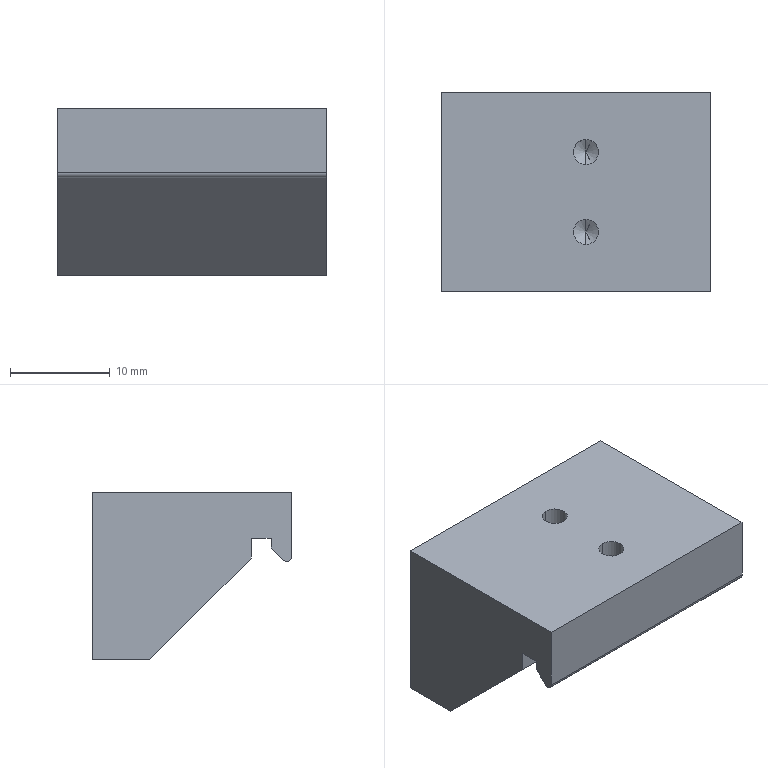Part | NX | 1 solid | 20 faces | box 27 x 20 x 16.8 mm | volume 6363 mm3 | plane 11 | cylinder 5 | cone 4 | commonest cylinder face diameters 2.5 x4 1 x1
STEP:
#1=CARTESIAN_POINT('',(1.,-5.25,-6.749));
#2=VERTEX_POINT('',#1);
#3=CARTESIAN_POINT('',(1.,-2.75,-6.749));
#4=VERTEX_POINT('',#3);
#5=CARTESIAN_POINT('',(1.,-4.,-6.749));
#6=DIRECTION('',(0.,0.,1.));
#7=DIRECTION('',(0.,1.,0.));
#8=AXIS2_PLACEMENT_3D('',#5,#6,#7);
#9=CIRCLE('',#8,1.25);
#10=EDGE_CURVE('',#2,#4,#9,.T.);
#11=ORIENTED_EDGE('',*,*,#10,.F.);
#12=CARTESIAN_POINT('',(1.,-5.25,0.));
#13=VERTEX_POINT('',#12);
#14=CARTESIAN_POINT('',(1.,-5.25,0.));
#15=DIRECTION('',(0.,0.,1.));
#16=VECTOR('',#15,1000.);
#17=LINE('',#14,#16);
#18=EDGE_CURVE('',#13,#2,#17,.F.);
#19=ORIENTED_EDGE('',*,*,#18,.F.);
#20=CARTESIAN_POINT('',(1.,-2.75,0.));
#21=VERTEX_POINT('',#20);
#22=CARTESIAN_POINT('',(1.,-4.,0.));
#23=DIRECTION('',(0.,0.,1.));
#24=DIRECTION('',(0.,1.,0.));
#25=AXIS2_PLACEMENT_3D('',#22,#23,#24);
#26=CIRCLE('',#25,1.25);
#27=EDGE_CURVE('',#13,#21,#26,.T.);
#28=ORIENTED_EDGE('',*,*,#27,.T.);
#29=CARTESIAN_POINT('',(1.,-2.75,0.));
#30=DIRECTION('',(0.,0.,1.));
#31=VECTOR('',#30,1000.);
#32=LINE('',#29,#31);
#33=EDGE_CURVE('',#21,#4,#32,.F.);
#34=ORIENTED_EDGE('',*,*,#33,.T.);
#35=EDGE_LOOP('',(#11,#19,#28,#34));
#36=FACE_BOUND('',#35,.T.);
#37=CARTESIAN_POINT('',(1.,-4.,0.));
#38=DIRECTION('',(0.,0.,1.));
#39=DIRECTION('',(0.,-1.,0.));
#40=AXIS2_PLACEMENT_3D('',#37,#38,#39);
#41=CYLINDRICAL_SURFACE('',#40,1.25);
#42=ADVANCED_FACE('',(#36),#41,.F.);
#43=CARTESIAN_POINT('',(1.,-4.,-7.5));
#44=VERTEX_POINT('',#43);
#45=CARTESIAN_POINT('',(1.,-2.75,-6.749));
#46=DIRECTION('',(0.,0.8572,0.515));
#47=VECTOR('',#46,1000.);
#48=LINE('',#45,#47);
#49=EDGE_CURVE('',#4,#44,#48,.F.);
#50=ORIENTED_EDGE('',*,*,#49,.T.);
#51=CARTESIAN_POINT('',(1.,-5.25,-6.749));
#52=DIRECTION('',(0.,-0.8572,0.515));
#53=VECTOR('',#52,1000.);
#54=LINE('',#51,#53);
#55=EDGE_CURVE('',#2,#44,#54,.F.);
#56=ORIENTED_EDGE('',*,*,#55,.F.);
#57=ORIENTED_EDGE('',*,*,#10,.T.);
#58=EDGE_LOOP('',(#50,#56,#57));
#59=FACE_BOUND('',#58,.T.);
#60=CARTESIAN_POINT('',(1.,-4.,-6.749));
#61=DIRECTION('',(0.,0.,1.));
#62=DIRECTION('',(0.,-1.,0.));
#63=AXIS2_PLACEMENT_3D('',#60,#61,#62);
#64=CONICAL_SURFACE('',#63,1.25,1.03);
#65=ADVANCED_FACE('',(#59),#64,.F.);
#66=CARTESIAN_POINT('',(1.,2.75,-6.749));
#67=VERTEX_POINT('',#66);
#68=CARTESIAN_POINT('',(1.,5.25,-6.749));
#69=VERTEX_POINT('',#68);
#70=CARTESIAN_POINT('',(1.,4.,-6.749));
#71=DIRECTION('',(0.,0.,1.));
#72=DIRECTION('',(0.,1.,0.));
#73=AXIS2_PLACEMENT_3D('',#70,#71,#72);
#74=CIRCLE('',#73,1.25);
#75=EDGE_CURVE('',#67,#69,#74,.T.);
#76=ORIENTED_EDGE('',*,*,#75,.F.);
#77=CARTESIAN_POINT('',(1.,2.75,0.));
#78=VERTEX_POINT('',#77);
#79=CARTESIAN_POINT('',(1.,2.75,0.));
#80=DIRECTION('',(0.,0.,1.));
#81=VECTOR('',#80,1000.);
#82=LINE('',#79,#81);
#83=EDGE_CURVE('',#78,#67,#82,.F.);
#84=ORIENTED_EDGE('',*,*,#83,.F.);
#85=CARTESIAN_POINT('',(1.,5.25,0.));
#86=VERTEX_POINT('',#85);
#87=CARTESIAN_POINT('',(1.,4.,0.));
#88=DIRECTION('',(0.,0.,1.));
#89=DIRECTION('',(0.,1.,0.));
#90=AXIS2_PLACEMENT_3D('',#87,#88,#89);
#91=CIRCLE('',#90,1.25);
#92=EDGE_CURVE('',#78,#86,#91,.T.);
#93=ORIENTED_EDGE('',*,*,#92,.T.);
#94=CARTESIAN_POINT('',(1.,5.25,0.));
#95=DIRECTION('',(0.,0.,1.));
#96=VECTOR('',#95,1000.);
#97=LINE('',#94,#96);
#98=EDGE_CURVE('',#86,#69,#97,.F.);
#99=ORIENTED_EDGE('',*,*,#98,.T.);
#100=EDGE_LOOP('',(#76,#84,#93,#99));
#101=FACE_BOUND('',#100,.T.);
#102=CARTESIAN_POINT('',(1.,4.,0.));
#103=DIRECTION('',(0.,0.,1.));
#104=DIRECTION('',(0.,-1.,0.));
#105=AXIS2_PLACEMENT_3D('',#102,#103,#104);
#106=CYLINDRICAL_SURFACE('',#105,1.25);
#107=ADVANCED_FACE('',(#101),#106,.F.);
#108=CARTESIAN_POINT('',(1.,4.,-7.5));
#109=VERTEX_POINT('',#108);
#110=CARTESIAN_POINT('',(1.,5.25,-6.749));
#111=DIRECTION('',(0.,0.8572,0.515));
#112=VECTOR('',#111,1000.);
#113=LINE('',#110,#112);
#114=EDGE_CURVE('',#69,#109,#113,.F.);
#115=ORIENTED_EDGE('',*,*,#114,.T.);
#116=CARTESIAN_POINT('',(1.,2.75,-6.749));
#117=DIRECTION('',(0.,-0.8572,0.515));
#118=VECTOR('',#117,1000.);
#119=LINE('',#116,#118);
#120=EDGE_CURVE('',#67,#109,#119,.F.);
#121=ORIENTED_EDGE('',*,*,#120,.F.);
#122=ORIENTED_EDGE('',*,*,#75,.T.);
#123=EDGE_LOOP('',(#115,#121,#122));
#124=FACE_BOUND('',#123,.T.);
#125=CARTESIAN_POINT('',(1.,4.,-6.749));
#126=DIRECTION('',(0.,0.,1.));
#127=DIRECTION('',(0.,-1.,0.));
#128=AXIS2_PLACEMENT_3D('',#125,#126,#127);
#129=CONICAL_SURFACE('',#128,1.25,1.03);
#130=ADVANCED_FACE('',(#124),#129,.F.);
#131=CARTESIAN_POINT('',(-13.5,-9.146,-6.816));
#132=VERTEX_POINT('',#131);
#133=CARTESIAN_POINT('',(-13.5,-7.93,-5.6));
#134=VERTEX_POINT('',#133);
#135=CARTESIAN_POINT('',(-13.5,-7.43,-5.1));
#136=DIRECTION('',(0.,0.7071,0.7071));
#137=VECTOR('',#136,1000.);
#138=LINE('',#135,#137);
#139=EDGE_CURVE('',#132,#134,#138,.T.);
#140=ORIENTED_EDGE('',*,*,#139,.F.);
#141=CARTESIAN_POINT('',(-13.5,-10.,-6.463));
#142=VERTEX_POINT('',#141);
#143=CARTESIAN_POINT('',(-13.5,-9.5,-6.463));
#144=DIRECTION('',(-1.,0.,0.));
#145=DIRECTION('',(0.,-1.,0.));
#146=AXIS2_PLACEMENT_3D('',#143,#144,#145);
#147=CIRCLE('',#146,0.5);
#148=EDGE_CURVE('',#132,#142,#147,.T.);
#149=ORIENTED_EDGE('',*,*,#148,.T.);
#150=CARTESIAN_POINT('',(-13.5,-10.,0.));
#151=VERTEX_POINT('',#150);
#152=CARTESIAN_POINT('',(-13.5,-10.,-16.8));
#153=DIRECTION('',(0.,0.,1.));
#154=VECTOR('',#153,1000.);
#155=LINE('',#152,#154);
#156=EDGE_CURVE('',#142,#151,#155,.T.);
#157=ORIENTED_EDGE('',*,*,#156,.T.);
#158=CARTESIAN_POINT('',(-13.5,10.,0.));
#159=VERTEX_POINT('',#158);
#160=CARTESIAN_POINT('',(-13.5,10.,0.));
#161=DIRECTION('',(0.,1.,0.));
#162=VECTOR('',#161,1000.);
#163=LINE('',#160,#162);
#164=EDGE_CURVE('',#151,#159,#163,.T.);
#165=ORIENTED_EDGE('',*,*,#164,.T.);
#166=CARTESIAN_POINT('',(-13.5,10.,-16.8));
#167=VERTEX_POINT('',#166);
#168=CARTESIAN_POINT('',(-13.5,10.,-16.8));
#169=DIRECTION('',(0.,0.,1.));
#170=VECTOR('',#169,1000.);
#171=LINE('',#168,#170);
#172=EDGE_CURVE('',#167,#159,#171,.T.);
#173=ORIENTED_EDGE('',*,*,#172,.F.);
#174=CARTESIAN_POINT('',(-13.5,4.27,-16.8));
#175=VERTEX_POINT('',#174);
#176=CARTESIAN_POINT('',(-13.5,10.,-16.8));
#177=DIRECTION('',(0.,1.,0.));
#178=VECTOR('',#177,1000.);
#179=LINE('',#176,#178);
#180=EDGE_CURVE('',#175,#167,#179,.T.);
#181=ORIENTED_EDGE('',*,*,#180,.F.);
#182=CARTESIAN_POINT('',(-13.5,-5.93,-6.6));
#183=VERTEX_POINT('',#182);
#184=CARTESIAN_POINT('',(-13.5,-7.43,-5.1));
#185=DIRECTION('',(0.,0.7071,-0.7071));
#186=VECTOR('',#185,1000.);
#187=LINE('',#184,#186);
#188=EDGE_CURVE('',#183,#175,#187,.T.);
#189=ORIENTED_EDGE('',*,*,#188,.F.);
#190=CARTESIAN_POINT('',(-13.5,-5.93,-4.6));
#191=VERTEX_POINT('',#190);
#192=CARTESIAN_POINT('',(-13.5,-5.93,-4.6));
#193=DIRECTION('',(0.,0.,-1.));
#194=VECTOR('',#193,1000.);
#195=LINE('',#192,#194);
#196=EDGE_CURVE('',#191,#183,#195,.T.);
#197=ORIENTED_EDGE('',*,*,#196,.F.);
#198=CARTESIAN_POINT('',(-13.5,-7.93,-4.6));
#199=VERTEX_POINT('',#198);
#200=CARTESIAN_POINT('',(-13.5,-7.93,-4.6));
#201=DIRECTION('',(0.,1.,0.));
#202=VECTOR('',#201,1000.);
#203=LINE('',#200,#202);
#204=EDGE_CURVE('',#199,#191,#203,.T.);
#205=ORIENTED_EDGE('',*,*,#204,.F.);
#206=CARTESIAN_POINT('',(-13.5,-7.93,-5.6));
#207=DIRECTION('',(0.,0.,1.));
#208=VECTOR('',#207,1000.);
#209=LINE('',#206,#208);
#210=EDGE_CURVE('',#134,#199,#209,.T.);
#211=ORIENTED_EDGE('',*,*,#210,.F.);
#212=EDGE_LOOP('',(#140,#149,#157,#165,#173,#181,#189,#197,#205,#211));
#213=FACE_BOUND('',#212,.T.);
#214=CARTESIAN_POINT('',(-13.5,10.,-16.8));
#215=DIRECTION('',(1.,0.,0.));
#216=DIRECTION('',(0.,1.,0.));
#217=AXIS2_PLACEMENT_3D('',#214,#215,#216);
#218=PLANE('',#217);
#219=ADVANCED_FACE('',(#213),#218,.F.);
#220=CARTESIAN_POINT('',(13.5,10.,0.));
#221=VERTEX_POINT('',#220);
#222=CARTESIAN_POINT('',(13.5,10.,0.));
#223=DIRECTION('',(1.,0.,0.));
#224=VECTOR('',#223,1000.);
#225=LINE('',#222,#224);
#226=EDGE_CURVE('',#159,#221,#225,.T.);
#227=ORIENTED_EDGE('',*,*,#226,.T.);
#228=CARTESIAN_POINT('',(13.5,10.,-16.8));
#229=VERTEX_POINT('',#228);
#230=CARTESIAN_POINT('',(13.5,10.,-16.8));
#231=DIRECTION('',(0.,0.,1.));
#232=VECTOR('',#231,1000.);
#233=LINE('',#230,#232);
#234=EDGE_CURVE('',#229,#221,#233,.T.);
#235=ORIENTED_EDGE('',*,*,#234,.F.);
#236=CARTESIAN_POINT('',(13.5,10.,-16.8));
#237=DIRECTION('',(1.,0.,0.));
#238=VECTOR('',#237,1000.);
#239=LINE('',#236,#238);
#240=EDGE_CURVE('',#167,#229,#239,.T.);
#241=ORIENTED_EDGE('',*,*,#240,.F.);
#242=ORIENTED_EDGE('',*,*,#172,.T.);
#243=EDGE_LOOP('',(#227,#235,#241,#242));
#244=FACE_BOUND('',#243,.T.);
#245=CARTESIAN_POINT('',(13.5,10.,-16.8));
#246=DIRECTION('',(0.,-1.,0.));
#247=DIRECTION('',(1.,0.,0.));
#248=AXIS2_PLACEMENT_3D('',#245,#246,#247);
#249=PLANE('',#248);
#250=ADVANCED_FACE('',(#244),#249,.F.);
#251=CARTESIAN_POINT('',(13.5,-10.,-6.463));
#252=VERTEX_POINT('',#251);
#253=CARTESIAN_POINT('',(13.5,-10.,0.));
#254=VERTEX_POINT('',#253);
#255=CARTESIAN_POINT('',(13.5,-10.,-16.8));
#256=DIRECTION('',(0.,0.,1.));
#257=VECTOR('',#256,1000.);
#258=LINE('',#255,#257);
#259=EDGE_CURVE('',#252,#254,#258,.T.);
#260=ORIENTED_EDGE('',*,*,#259,.F.);
#261=CARTESIAN_POINT('',(13.5,-9.146,-6.816));
#262=VERTEX_POINT('',#261);
#263=CARTESIAN_POINT('',(13.5,-9.5,-6.463));
#264=DIRECTION('',(1.,0.,0.));
#265=DIRECTION('',(0.,1.,0.));
#266=AXIS2_PLACEMENT_3D('',#263,#264,#265);
#267=CIRCLE('',#266,0.5);
#268=EDGE_CURVE('',#252,#262,#267,.T.);
#269=ORIENTED_EDGE('',*,*,#268,.T.);
#270=CARTESIAN_POINT('',(13.5,-7.93,-5.6));
#271=VERTEX_POINT('',#270);
#272=CARTESIAN_POINT('',(13.5,-7.43,-5.1));
#273=DIRECTION('',(0.,0.7071,0.7071));
#274=VECTOR('',#273,1000.);
#275=LINE('',#272,#274);
#276=EDGE_CURVE('',#262,#271,#275,.T.);
#277=ORIENTED_EDGE('',*,*,#276,.T.);
#278=CARTESIAN_POINT('',(13.5,-7.93,-4.6));
#279=VERTEX_POINT('',#278);
#280=CARTESIAN_POINT('',(13.5,-7.93,-5.6));
#281=DIRECTION('',(0.,0.,1.));
#282=VECTOR('',#281,1000.);
#283=LINE('',#280,#282);
#284=EDGE_CURVE('',#271,#279,#283,.T.);
#285=ORIENTED_EDGE('',*,*,#284,.T.);
#286=CARTESIAN_POINT('',(13.5,-5.93,-4.6));
#287=VERTEX_POINT('',#286);
#288=CARTESIAN_POINT('',(13.5,-7.93,-4.6));
#289=DIRECTION('',(0.,1.,0.));
#290=VECTOR('',#289,1000.);
#291=LINE('',#288,#290);
#292=EDGE_CURVE('',#279,#287,#291,.T.);
#293=ORIENTED_EDGE('',*,*,#292,.T.);
#294=CARTESIAN_POINT('',(13.5,-5.93,-6.6));
#295=VERTEX_POINT('',#294);
#296=CARTESIAN_POINT('',(13.5,-5.93,-16.8));
#297=DIRECTION('',(0.,0.,-1.));
#298=VECTOR('',#297,1000.);
#299=LINE('',#296,#298);
#300=EDGE_CURVE('',#287,#295,#299,.T.);
#301=ORIENTED_EDGE('',*,*,#300,.T.);
#302=CARTESIAN_POINT('',(13.5,4.27,-16.8));
#303=VERTEX_POINT('',#302);
#304=CARTESIAN_POINT('',(13.5,-7.43,-5.1));
#305=DIRECTION('',(0.,0.7071,-0.7071));
#306=VECTOR('',#305,1000.);
#307=LINE('',#304,#306);
#308=EDGE_CURVE('',#295,#303,#307,.T.);
#309=ORIENTED_EDGE('',*,*,#308,.T.);
#310=CARTESIAN_POINT('',(13.5,10.,-16.8));
#311=DIRECTION('',(0.,-1.,0.));
#312=VECTOR('',#311,1000.);
#313=LINE('',#310,#312);
#314=EDGE_CURVE('',#229,#303,#313,.T.);
#315=ORIENTED_EDGE('',*,*,#314,.F.);
#316=ORIENTED_EDGE('',*,*,#234,.T.);
#317=CARTESIAN_POINT('',(13.5,10.,0.));
#318=DIRECTION('',(0.,-1.,0.));
#319=VECTOR('',#318,1000.);
#320=LINE('',#317,#319);
#321=EDGE_CURVE('',#221,#254,#320,.T.);
#322=ORIENTED_EDGE('',*,*,#321,.T.);
#323=EDGE_LOOP('',(#260,#269,#277,#285,#293,#301,#309,#315,#316,#322));
#324=FACE_BOUND('',#323,.T.);
#325=CARTESIAN_POINT('',(13.5,10.,-16.8));
#326=DIRECTION('',(-1.,0.,0.));
#327=DIRECTION('',(0.,-1.,0.));
#328=AXIS2_PLACEMENT_3D('',#325,#326,#327);
#329=PLANE('',#328);
#330=ADVANCED_FACE('',(#324),#329,.F.);
#331=ORIENTED_EDGE('',*,*,#156,.F.);
#332=CARTESIAN_POINT('',(13.5,-10.,-6.463));
#333=DIRECTION('',(1.,0.,0.));
#334=VECTOR('',#333,1000.);
#335=LINE('',#332,#334);
#336=EDGE_CURVE('',#142,#252,#335,.T.);
#337=ORIENTED_EDGE('',*,*,#336,.T.);
#338=ORIENTED_EDGE('',*,*,#259,.T.);
#339=CARTESIAN_POINT('',(13.5,-10.,0.));
#340=DIRECTION('',(-1.,0.,0.));
#341=VECTOR('',#340,1000.);
#342=LINE('',#339,#341);
#343=EDGE_CURVE('',#254,#151,#342,.T.);
#344=ORIENTED_EDGE('',*,*,#343,.T.);
#345=EDGE_LOOP('',(#331,#337,#338,#344));
#346=FACE_BOUND('',#345,.T.);
#347=CARTESIAN_POINT('',(13.5,-10.,-16.8));
#348=DIRECTION('',(0.,1.,0.));
#349=DIRECTION('',(-1.,0.,0.));
#350=AXIS2_PLACEMENT_3D('',#347,#348,#349);
#351=PLANE('',#350);
#352=ADVANCED_FACE('',(#346),#351,.F.);
#353=CARTESIAN_POINT('',(13.5,4.27,-16.8));
#354=DIRECTION('',(-1.,0.,0.));
#355=VECTOR('',#354,1000.);
#356=LINE('',#353,#355);
#357=EDGE_CURVE('',#303,#175,#356,.T.);
#358=ORIENTED_EDGE('',*,*,#357,.T.);
#359=ORIENTED_EDGE('',*,*,#180,.T.);
#360=ORIENTED_EDGE('',*,*,#240,.T.);
#361=ORIENTED_EDGE('',*,*,#314,.T.);
#362=EDGE_LOOP('',(#358,#359,#360,#361));
#363=FACE_BOUND('',#362,.T.);
#364=CARTESIAN_POINT('',(0.,0.,-16.8));
#365=DIRECTION('',(0.,0.,-1.));
#366=DIRECTION('',(0.,1.,0.));
#367=AXIS2_PLACEMENT_3D('',#364,#365,#366);
#368=PLANE('',#367);
#369=ADVANCED_FACE('',(#363),#368,.T.);
#370=CARTESIAN_POINT('',(1.,-4.,0.));
#371=DIRECTION('',(0.,0.,1.));
#372=DIRECTION('',(0.,1.,0.));
#373=AXIS2_PLACEMENT_3D('',#370,#371,#372);
#374=CIRCLE('',#373,1.25);
#375=EDGE_CURVE('',#21,#13,#374,.T.);
#376=ORIENTED_EDGE('',*,*,#375,.F.);
#377=ORIENTED_EDGE('',*,*,#27,.F.);
#378=EDGE_LOOP('',(#376,#377));
#379=FACE_BOUND('',#378,.T.);
#380=CARTESIAN_POINT('',(1.,4.,0.));
#381=DIRECTION('',(0.,0.,1.));
#382=DIRECTION('',(0.,1.,0.));
#383=AXIS2_PLACEMENT_3D('',#380,#381,#382);
#384=CIRCLE('',#383,1.25);
#385=EDGE_CURVE('',#86,#78,#384,.T.);
#386=ORIENTED_EDGE('',*,*,#385,.F.);
#387=ORIENTED_EDGE('',*,*,#92,.F.);
#388=EDGE_LOOP('',(#386,#387));
#389=FACE_BOUND('',#388,.T.);
#390=ORIENTED_EDGE('',*,*,#164,.F.);
#391=ORIENTED_EDGE('',*,*,#343,.F.);
#392=ORIENTED_EDGE('',*,*,#321,.F.);
#393=ORIENTED_EDGE('',*,*,#226,.F.);
#394=EDGE_LOOP('',(#390,#391,#392,#393));
#395=FACE_BOUND('',#394,.T.);
#396=CARTESIAN_POINT('',(0.,0.,0.));
#397=DIRECTION('',(0.,0.,-1.));
#398=DIRECTION('',(0.,1.,0.));
#399=AXIS2_PLACEMENT_3D('',#396,#397,#398);
#400=PLANE('',#399);
#401=ADVANCED_FACE('',(#379,#389,#395),#400,.F.);
#402=ORIENTED_EDGE('',*,*,#308,.F.);
#403=CARTESIAN_POINT('',(13.5,-5.93,-6.6));
#404=DIRECTION('',(-1.,0.,0.));
#405=VECTOR('',#404,1000.);
#406=LINE('',#403,#405);
#407=EDGE_CURVE('',#295,#183,#406,.T.);
#408=ORIENTED_EDGE('',*,*,#407,.T.);
#409=ORIENTED_EDGE('',*,*,#188,.T.);
#410=ORIENTED_EDGE('',*,*,#357,.F.);
#411=EDGE_LOOP('',(#402,#408,#409,#410));
#412=FACE_BOUND('',#411,.T.);
#413=CARTESIAN_POINT('',(13.5,-7.43,-5.1));
#414=DIRECTION('',(0.,0.7071,0.7071));
#415=DIRECTION('',(0.,-0.7071,0.7071));
#416=AXIS2_PLACEMENT_3D('',#413,#414,#415);
#417=PLANE('',#416);
#418=ADVANCED_FACE('',(#412),#417,.F.);
#419=ORIENTED_EDGE('',*,*,#276,.F.);
#420=CARTESIAN_POINT('',(13.5,-9.146,-6.816));
#421=DIRECTION('',(-1.,0.,0.));
#422=VECTOR('',#421,1000.);
#423=LINE('',#420,#422);
#424=EDGE_CURVE('',#262,#132,#423,.T.);
#425=ORIENTED_EDGE('',*,*,#424,.T.);
#426=ORIENTED_EDGE('',*,*,#139,.T.);
#427=CARTESIAN_POINT('',(13.5,-7.93,-5.6));
#428=DIRECTION('',(-1.,0.,0.));
#429=VECTOR('',#428,1000.);
#430=LINE('',#427,#429);
#431=EDGE_CURVE('',#271,#134,#430,.T.);
#432=ORIENTED_EDGE('',*,*,#431,.F.);
#433=EDGE_LOOP('',(#419,#425,#426,#432));
#434=FACE_BOUND('',#433,.T.);
#435=CARTESIAN_POINT('',(13.5,-7.43,-5.1));
#436=DIRECTION('',(0.,-0.7071,0.7071));
#437=DIRECTION('',(0.,-0.7071,-0.7071));
#438=AXIS2_PLACEMENT_3D('',#435,#436,#437);
#439=PLANE('',#438);
#440=ADVANCED_FACE('',(#434),#439,.F.);
#441=ORIENTED_EDGE('',*,*,#196,.T.);
#442=ORIENTED_EDGE('',*,*,#407,.F.);
#443=ORIENTED_EDGE('',*,*,#300,.F.);
#444=CARTESIAN_POINT('',(13.5,-5.93,-4.6));
#445=DIRECTION('',(-1.,0.,0.));
#446=VECTOR('',#445,1000.);
#447=LINE('',#444,#446);
#448=EDGE_CURVE('',#287,#191,#447,.T.);
#449=ORIENTED_EDGE('',*,*,#448,.T.);
#450=EDGE_LOOP('',(#441,#442,#443,#449));
#451=FACE_BOUND('',#450,.T.);
#452=CARTESIAN_POINT('',(13.5,-5.93,-4.6));
#453=DIRECTION('',(0.,1.,0.));
#454=DIRECTION('',(0.,0.,1.));
#455=AXIS2_PLACEMENT_3D('',#452,#453,#454);
#456=PLANE('',#455);
#457=ADVANCED_FACE('',(#451),#456,.F.);
#458=ORIENTED_EDGE('',*,*,#204,.T.);
#459=ORIENTED_EDGE('',*,*,#448,.F.);
#460=ORIENTED_EDGE('',*,*,#292,.F.);
#461=CARTESIAN_POINT('',(13.5,-7.93,-4.6));
#462=DIRECTION('',(-1.,0.,0.));
#463=VECTOR('',#462,1000.);
#464=LINE('',#461,#463);
#465=EDGE_CURVE('',#279,#199,#464,.T.);
#466=ORIENTED_EDGE('',*,*,#465,.T.);
#467=EDGE_LOOP('',(#458,#459,#460,#466));
#468=FACE_BOUND('',#467,.T.);
#469=CARTESIAN_POINT('',(13.5,-7.93,-4.6));
#470=DIRECTION('',(0.,0.,1.));
#471=DIRECTION('',(0.,-1.,0.));
#472=AXIS2_PLACEMENT_3D('',#469,#470,#471);
#473=PLANE('',#472);
#474=ADVANCED_FACE('',(#468),#473,.F.);
#475=ORIENTED_EDGE('',*,*,#210,.T.);
#476=ORIENTED_EDGE('',*,*,#465,.F.);
#477=ORIENTED_EDGE('',*,*,#284,.F.);
#478=ORIENTED_EDGE('',*,*,#431,.T.);
#479=EDGE_LOOP('',(#475,#476,#477,#478));
#480=FACE_BOUND('',#479,.T.);
#481=CARTESIAN_POINT('',(13.5,-7.93,-5.6));
#482=DIRECTION('',(0.,-1.,0.));
#483=DIRECTION('',(0.,0.,-1.));
#484=AXIS2_PLACEMENT_3D('',#481,#482,#483);
#485=PLANE('',#484);
#486=ADVANCED_FACE('',(#480),#485,.F.);
#487=ORIENTED_EDGE('',*,*,#268,.F.);
#488=ORIENTED_EDGE('',*,*,#336,.F.);
#489=ORIENTED_EDGE('',*,*,#148,.F.);
#490=ORIENTED_EDGE('',*,*,#424,.F.);
#491=EDGE_LOOP('',(#487,#488,#489,#490));
#492=FACE_BOUND('',#491,.T.);
#493=CARTESIAN_POINT('',(13.5,-9.5,-6.463));
#494=DIRECTION('',(-1.,0.,0.));
#495=DIRECTION('',(0.,-1.,0.));
#496=AXIS2_PLACEMENT_3D('',#493,#494,#495);
#497=CYLINDRICAL_SURFACE('',#496,0.5);
#498=ADVANCED_FACE('',(#492),#497,.T.);
#499=ORIENTED_EDGE('',*,*,#120,.T.);
#500=ORIENTED_EDGE('',*,*,#114,.F.);
#501=CARTESIAN_POINT('',(1.,4.,-6.749));
#502=DIRECTION('',(0.,0.,1.));
#503=DIRECTION('',(0.,1.,0.));
#504=AXIS2_PLACEMENT_3D('',#501,#502,#503);
#505=CIRCLE('',#504,1.25);
#506=EDGE_CURVE('',#69,#67,#505,.T.);
#507=ORIENTED_EDGE('',*,*,#506,.T.);
#508=EDGE_LOOP('',(#499,#500,#507));
#509=FACE_BOUND('',#508,.T.);
#510=CARTESIAN_POINT('',(1.,4.,-6.749));
#511=DIRECTION('',(0.,0.,1.));
#512=DIRECTION('',(0.,-1.,0.));
#513=AXIS2_PLACEMENT_3D('',#510,#511,#512);
#514=CONICAL_SURFACE('',#513,1.25,1.03);
#515=ADVANCED_FACE('',(#509),#514,.F.);
#516=ORIENTED_EDGE('',*,*,#83,.T.);
#517=ORIENTED_EDGE('',*,*,#506,.F.);
#518=ORIENTED_EDGE('',*,*,#98,.F.);
#519=ORIENTED_EDGE('',*,*,#385,.T.);
#520=EDGE_LOOP('',(#516,#517,#518,#519));
#521=FACE_BOUND('',#520,.T.);
#522=CARTESIAN_POINT('',(1.,4.,0.));
#523=DIRECTION('',(0.,0.,1.));
#524=DIRECTION('',(0.,-1.,0.));
#525=AXIS2_PLACEMENT_3D('',#522,#523,#524);
#526=CYLINDRICAL_SURFACE('',#525,1.25);
#527=ADVANCED_FACE('',(#521),#526,.F.);
#528=ORIENTED_EDGE('',*,*,#55,.T.);
#529=ORIENTED_EDGE('',*,*,#49,.F.);
#530=CARTESIAN_POINT('',(1.,-4.,-6.749));
#531=DIRECTION('',(0.,0.,1.));
#532=DIRECTION('',(0.,1.,0.));
#533=AXIS2_PLACEMENT_3D('',#530,#531,#532);
#534=CIRCLE('',#533,1.25);
#535=EDGE_CURVE('',#4,#2,#534,.T.);
#536=ORIENTED_EDGE('',*,*,#535,.T.);
#537=EDGE_LOOP('',(#528,#529,#536));
#538=FACE_BOUND('',#537,.T.);
#539=CARTESIAN_POINT('',(1.,-4.,-6.749));
#540=DIRECTION('',(0.,0.,1.));
#541=DIRECTION('',(0.,-1.,0.));
#542=AXIS2_PLACEMENT_3D('',#539,#540,#541);
#543=CONICAL_SURFACE('',#542,1.25,1.03);
#544=ADVANCED_FACE('',(#538),#543,.F.);
#545=ORIENTED_EDGE('',*,*,#18,.T.);
#546=ORIENTED_EDGE('',*,*,#535,.F.);
#547=ORIENTED_EDGE('',*,*,#33,.F.);
#548=ORIENTED_EDGE('',*,*,#375,.T.);
#549=EDGE_LOOP('',(#545,#546,#547,#548));
#550=FACE_BOUND('',#549,.T.);
#551=CARTESIAN_POINT('',(1.,-4.,0.));
#552=DIRECTION('',(0.,0.,1.));
#553=DIRECTION('',(0.,-1.,0.));
#554=AXIS2_PLACEMENT_3D('',#551,#552,#553);
#555=CYLINDRICAL_SURFACE('',#554,1.25);
#556=ADVANCED_FACE('',(#550),#555,.F.);
#557=CLOSED_SHELL('',(#42,#65,#107,#130,#219,#250,#330,#352,#369,#401,#418,#440,#457,#474,#486,#498,#515,#527,#544,#556));
#558=MANIFOLD_SOLID_BREP('',#557);
#559=(LENGTH_UNIT()NAMED_UNIT(*)SI_UNIT(.MILLI.,.METRE.));
#560=UNCERTAINTY_MEASURE_WITH_UNIT(LENGTH_MEASURE(0.00001),#559,'','');
#561=(NAMED_UNIT(*)PLANE_ANGLE_UNIT()SI_UNIT($,.RADIAN.));
#562=(NAMED_UNIT(*)SI_UNIT($,.STERADIAN.)SOLID_ANGLE_UNIT());
#563=(GEOMETRIC_REPRESENTATION_CONTEXT(3)GLOBAL_UNCERTAINTY_ASSIGNED_CONTEXT((#560))GLOBAL_UNIT_ASSIGNED_CONTEXT((#559,#561,#562))REPRESENTATION_CONTEXT('',''));
#564=ADVANCED_BREP_SHAPE_REPRESENTATION('',(#558),#563);